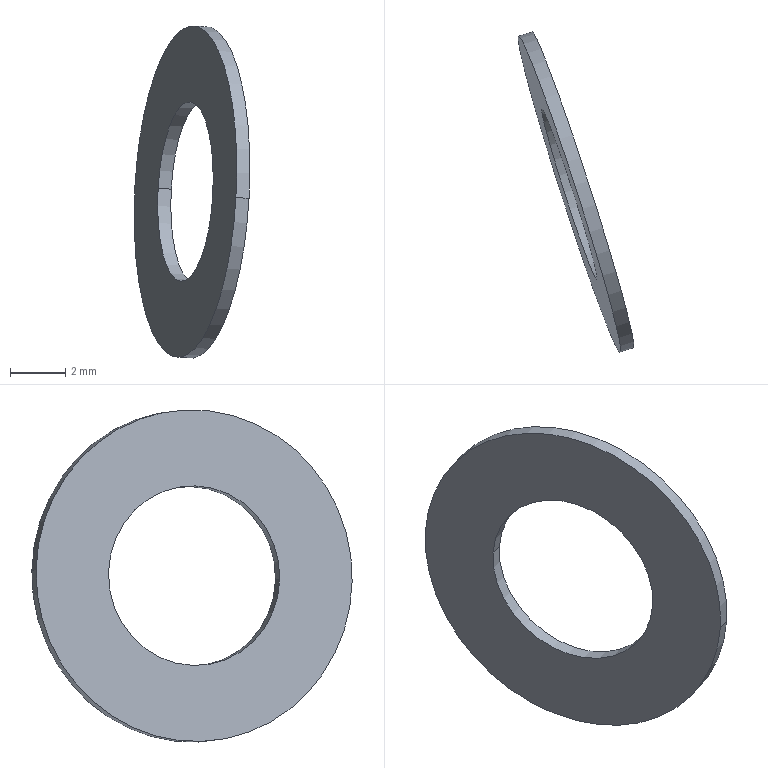Part | SolidWorks | features BaseBody 1 | 1 solid | 6 faces | box 4.184 x 11.579 x 12.01 mm | volume 39.957 mm3 | cylinder 4 | plane 2 | commonest cylinder face diameters 6.5 x2 12 x2
STEP:
#1=CARTESIAN_POINT('',(62.713,-71.369,-184.304));
#2=VERTEX_POINT('',#1);
#3=CARTESIAN_POINT('',(66.361,-82.793,-184.733));
#4=VERTEX_POINT('',#3);
#5=CARTESIAN_POINT('',(64.537,-77.081,-184.518));
#6=DIRECTION('',(-0.9511,-0.3055,0.04654));
#7=DIRECTION('',(-0.304,0.952,0.03578));
#8=AXIS2_PLACEMENT_3D('',#5,#6,#7);
#9=CIRCLE('',#8,6.);
#10=EDGE_CURVE('',#2,#4,#9,.T.);
#11=ORIENTED_EDGE('',*,*,#10,.F.);
#12=CARTESIAN_POINT('',(63.188,-71.217,-184.327));
#13=VERTEX_POINT('',#12);
#14=CARTESIAN_POINT('',(62.713,-71.369,-184.304));
#15=DIRECTION('',(0.9511,0.3055,-0.04654));
#16=VECTOR('',#15,1000.);
#17=LINE('',#14,#16);
#18=EDGE_CURVE('',#2,#13,#17,.T.);
#19=ORIENTED_EDGE('',*,*,#18,.T.);
#20=CARTESIAN_POINT('',(66.837,-82.64,-184.756));
#21=VERTEX_POINT('',#20);
#22=CARTESIAN_POINT('',(65.013,-76.928,-184.542));
#23=DIRECTION('',(-0.9511,-0.3055,0.04654));
#24=DIRECTION('',(-0.304,0.952,0.03578));
#25=AXIS2_PLACEMENT_3D('',#22,#23,#24);
#26=CIRCLE('',#25,6.);
#27=EDGE_CURVE('',#13,#21,#26,.T.);
#28=ORIENTED_EDGE('',*,*,#27,.T.);
#29=CARTESIAN_POINT('',(66.361,-82.793,-184.733));
#30=DIRECTION('',(0.9511,0.3055,-0.04654));
#31=VECTOR('',#30,1000.);
#32=LINE('',#29,#31);
#33=EDGE_CURVE('',#4,#21,#32,.T.);
#34=ORIENTED_EDGE('',*,*,#33,.F.);
#35=EDGE_LOOP('',(#11,#19,#28,#34));
#36=FACE_OUTER_BOUND('',#35,.T.);
#37=CARTESIAN_POINT('',(64.537,-77.081,-184.518));
#38=DIRECTION('',(0.9511,0.3055,-0.04654));
#39=DIRECTION('',(0.304,-0.952,-0.03578));
#40=AXIS2_PLACEMENT_3D('',#37,#38,#39);
#41=CYLINDRICAL_SURFACE('',#40,6.);
#42=ADVANCED_FACE('',(#36),#41,.T.);
#43=CARTESIAN_POINT('',(65.525,-80.175,-184.635));
#44=VERTEX_POINT('',#43);
#45=CARTESIAN_POINT('',(63.549,-73.987,-184.402));
#46=VERTEX_POINT('',#45);
#47=CARTESIAN_POINT('',(64.537,-77.081,-184.518));
#48=DIRECTION('',(-0.9511,-0.3055,0.04654));
#49=DIRECTION('',(-0.304,0.952,0.03578));
#50=AXIS2_PLACEMENT_3D('',#47,#48,#49);
#51=CIRCLE('',#50,3.25);
#52=EDGE_CURVE('',#44,#46,#51,.T.);
#53=ORIENTED_EDGE('',*,*,#52,.T.);
#54=CARTESIAN_POINT('',(64.024,-73.835,-184.425));
#55=VERTEX_POINT('',#54);
#56=CARTESIAN_POINT('',(63.549,-73.987,-184.402));
#57=DIRECTION('',(0.9511,0.3055,-0.04654));
#58=VECTOR('',#57,1000.);
#59=LINE('',#56,#58);
#60=EDGE_CURVE('',#46,#55,#59,.T.);
#61=ORIENTED_EDGE('',*,*,#60,.T.);
#62=CARTESIAN_POINT('',(66.001,-80.022,-184.658));
#63=VERTEX_POINT('',#62);
#64=CARTESIAN_POINT('',(65.013,-76.928,-184.542));
#65=DIRECTION('',(-0.9511,-0.3055,0.04654));
#66=DIRECTION('',(-0.304,0.952,0.03578));
#67=AXIS2_PLACEMENT_3D('',#64,#65,#66);
#68=CIRCLE('',#67,3.25);
#69=EDGE_CURVE('',#63,#55,#68,.T.);
#70=ORIENTED_EDGE('',*,*,#69,.F.);
#71=CARTESIAN_POINT('',(65.525,-80.175,-184.635));
#72=DIRECTION('',(0.9511,0.3055,-0.04654));
#73=VECTOR('',#72,1000.);
#74=LINE('',#71,#73);
#75=EDGE_CURVE('',#44,#63,#74,.T.);
#76=ORIENTED_EDGE('',*,*,#75,.F.);
#77=EDGE_LOOP('',(#53,#61,#70,#76));
#78=FACE_OUTER_BOUND('',#77,.T.);
#79=CARTESIAN_POINT('',(64.537,-77.081,-184.518));
#80=DIRECTION('',(0.9511,0.3055,-0.04654));
#81=DIRECTION('',(0.304,-0.952,-0.03578));
#82=AXIS2_PLACEMENT_3D('',#79,#80,#81);
#83=CYLINDRICAL_SURFACE('',#82,3.25);
#84=ADVANCED_FACE('',(#78),#83,.F.);
#85=ORIENTED_EDGE('',*,*,#60,.F.);
#86=CARTESIAN_POINT('',(64.537,-77.081,-184.518));
#87=DIRECTION('',(-0.9511,-0.3055,0.04654));
#88=DIRECTION('',(-0.304,0.952,0.03578));
#89=AXIS2_PLACEMENT_3D('',#86,#87,#88);
#90=CIRCLE('',#89,3.25);
#91=EDGE_CURVE('',#46,#44,#90,.T.);
#92=ORIENTED_EDGE('',*,*,#91,.T.);
#93=ORIENTED_EDGE('',*,*,#75,.T.);
#94=CARTESIAN_POINT('',(65.013,-76.928,-184.542));
#95=DIRECTION('',(-0.9511,-0.3055,0.04654));
#96=DIRECTION('',(-0.304,0.952,0.03578));
#97=AXIS2_PLACEMENT_3D('',#94,#95,#96);
#98=CIRCLE('',#97,3.25);
#99=EDGE_CURVE('',#55,#63,#98,.T.);
#100=ORIENTED_EDGE('',*,*,#99,.F.);
#101=EDGE_LOOP('',(#85,#92,#93,#100));
#102=FACE_OUTER_BOUND('',#101,.T.);
#103=CARTESIAN_POINT('',(64.537,-77.081,-184.518));
#104=DIRECTION('',(0.9511,0.3055,-0.04654));
#105=DIRECTION('',(0.304,-0.952,-0.03578));
#106=AXIS2_PLACEMENT_3D('',#103,#104,#105);
#107=CYLINDRICAL_SURFACE('',#106,3.25);
#108=ADVANCED_FACE('',(#102),#107,.F.);
#109=ORIENTED_EDGE('',*,*,#18,.F.);
#110=CARTESIAN_POINT('',(64.537,-77.081,-184.518));
#111=DIRECTION('',(-0.9511,-0.3055,0.04654));
#112=DIRECTION('',(-0.304,0.952,0.03578));
#113=AXIS2_PLACEMENT_3D('',#110,#111,#112);
#114=CIRCLE('',#113,6.);
#115=EDGE_CURVE('',#4,#2,#114,.T.);
#116=ORIENTED_EDGE('',*,*,#115,.F.);
#117=ORIENTED_EDGE('',*,*,#33,.T.);
#118=CARTESIAN_POINT('',(65.013,-76.928,-184.542));
#119=DIRECTION('',(-0.9511,-0.3055,0.04654));
#120=DIRECTION('',(-0.304,0.952,0.03578));
#121=AXIS2_PLACEMENT_3D('',#118,#119,#120);
#122=CIRCLE('',#121,6.);
#123=EDGE_CURVE('',#21,#13,#122,.T.);
#124=ORIENTED_EDGE('',*,*,#123,.T.);
#125=EDGE_LOOP('',(#109,#116,#117,#124));
#126=FACE_OUTER_BOUND('',#125,.T.);
#127=CARTESIAN_POINT('',(64.537,-77.081,-184.518));
#128=DIRECTION('',(0.9511,0.3055,-0.04654));
#129=DIRECTION('',(0.304,-0.952,-0.03578));
#130=AXIS2_PLACEMENT_3D('',#127,#128,#129);
#131=CYLINDRICAL_SURFACE('',#130,6.);
#132=ADVANCED_FACE('',(#126),#131,.T.);
#133=ORIENTED_EDGE('',*,*,#69,.T.);
#134=ORIENTED_EDGE('',*,*,#99,.T.);
#135=EDGE_LOOP('',(#133,#134));
#136=FACE_BOUND('',#135,.T.);
#137=ORIENTED_EDGE('',*,*,#123,.F.);
#138=ORIENTED_EDGE('',*,*,#27,.F.);
#139=EDGE_LOOP('',(#137,#138));
#140=FACE_OUTER_BOUND('',#139,.T.);
#141=CARTESIAN_POINT('',(65.013,-76.928,-184.542));
#142=DIRECTION('',(-0.9511,-0.3055,0.04654));
#143=DIRECTION('',(-0.3058,0.9521,0.));
#144=AXIS2_PLACEMENT_3D('',#141,#142,#143);
#145=PLANE('',#144);
#146=ADVANCED_FACE('',(#136,#140),#145,.F.);
#147=ORIENTED_EDGE('',*,*,#52,.F.);
#148=ORIENTED_EDGE('',*,*,#91,.F.);
#149=EDGE_LOOP('',(#147,#148));
#150=FACE_BOUND('',#149,.T.);
#151=ORIENTED_EDGE('',*,*,#115,.T.);
#152=ORIENTED_EDGE('',*,*,#10,.T.);
#153=EDGE_LOOP('',(#151,#152));
#154=FACE_OUTER_BOUND('',#153,.T.);
#155=CARTESIAN_POINT('',(64.537,-77.081,-184.518));
#156=DIRECTION('',(-0.9511,-0.3055,0.04654));
#157=DIRECTION('',(-0.3058,0.9521,0.));
#158=AXIS2_PLACEMENT_3D('',#155,#156,#157);
#159=PLANE('',#158);
#160=ADVANCED_FACE('',(#150,#154),#159,.T.);
#161=CLOSED_SHELL('',(#42,#84,#108,#132,#146,#160));
#162=MANIFOLD_SOLID_BREP('',#161);
#163=CARTESIAN_POINT('',(0.,0.,0.));
#164=DIRECTION('',(0.,0.,1.));
#165=DIRECTION('',(1.,0.,0.));
#166=AXIS2_PLACEMENT_3D('',#163,#164,#165);
#167=(LENGTH_UNIT()NAMED_UNIT(*)SI_UNIT(.MILLI.,.METRE.));
#168=UNCERTAINTY_MEASURE_WITH_UNIT(LENGTH_MEASURE(0.00001),#167,'','');
#169=(NAMED_UNIT(*)PLANE_ANGLE_UNIT()SI_UNIT($,.RADIAN.));
#170=(NAMED_UNIT(*)SI_UNIT($,.STERADIAN.)SOLID_ANGLE_UNIT());
#171=(GEOMETRIC_REPRESENTATION_CONTEXT(3)GLOBAL_UNCERTAINTY_ASSIGNED_CONTEXT((#168))GLOBAL_UNIT_ASSIGNED_CONTEXT((#167,#169,#170))REPRESENTATION_CONTEXT('',''));
#172=ADVANCED_BREP_SHAPE_REPRESENTATION('',(#162,#166),#171);